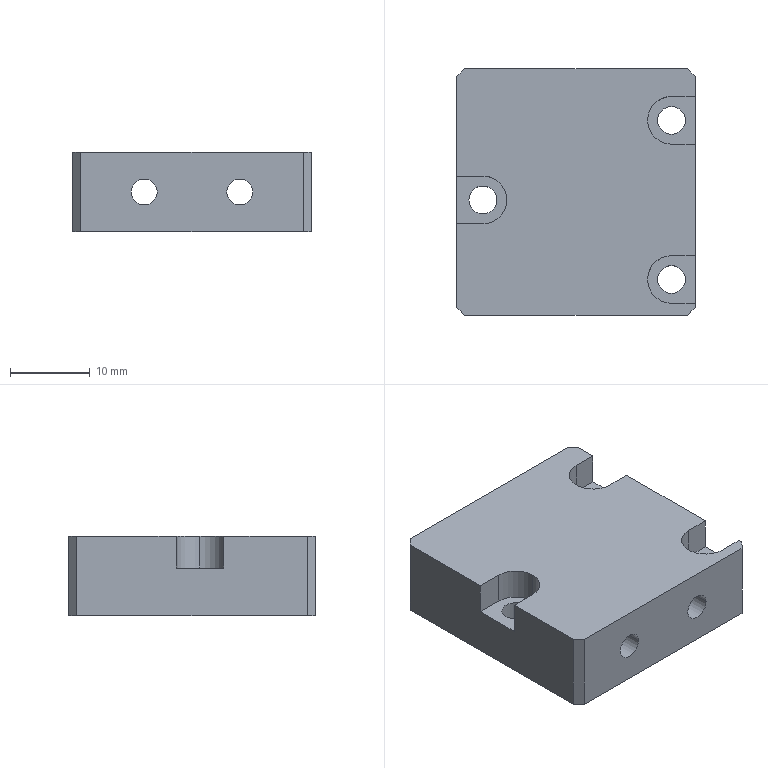Part | STEP file | ASND-0110-Body 1-18 | 1 solid | 33 faces | box 30 x 31 x 10 mm | volume 8202 mm3 | plane 19 | cylinder 14 | commonest cylinder face diameters 3.5 x6 3.242 x4 6 x4